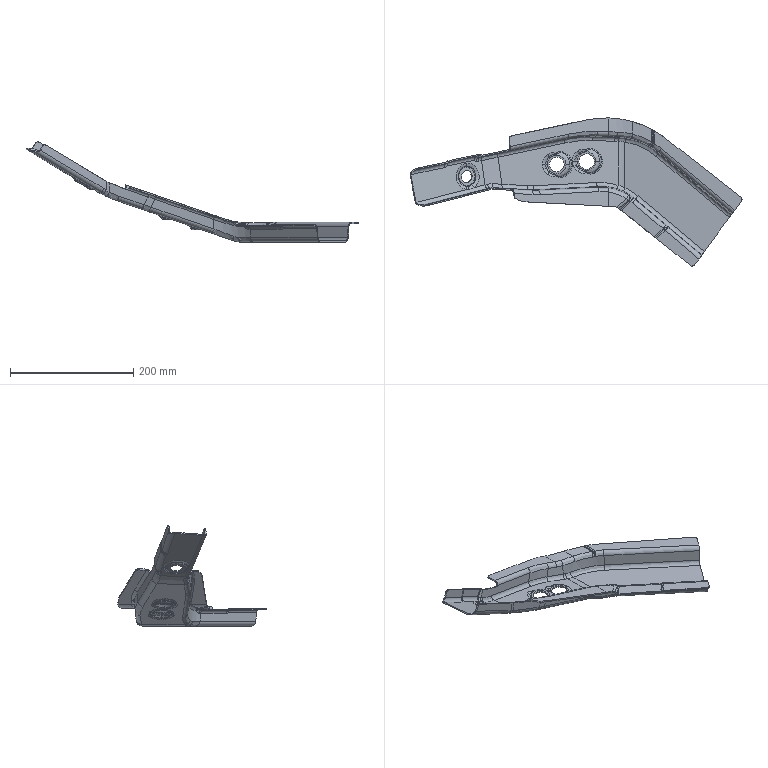Part | 1 solid | 363 faces | box 538.98 x 240.546 x 162.508 mm | volume 165586 mm3 | spline 245 | cylinder 74 | plane 36 | sphere 4 | other 4 | commonest cylinder face diameters 10 x14 13 x11 17 x10 14 x9 6 x3 20 x2